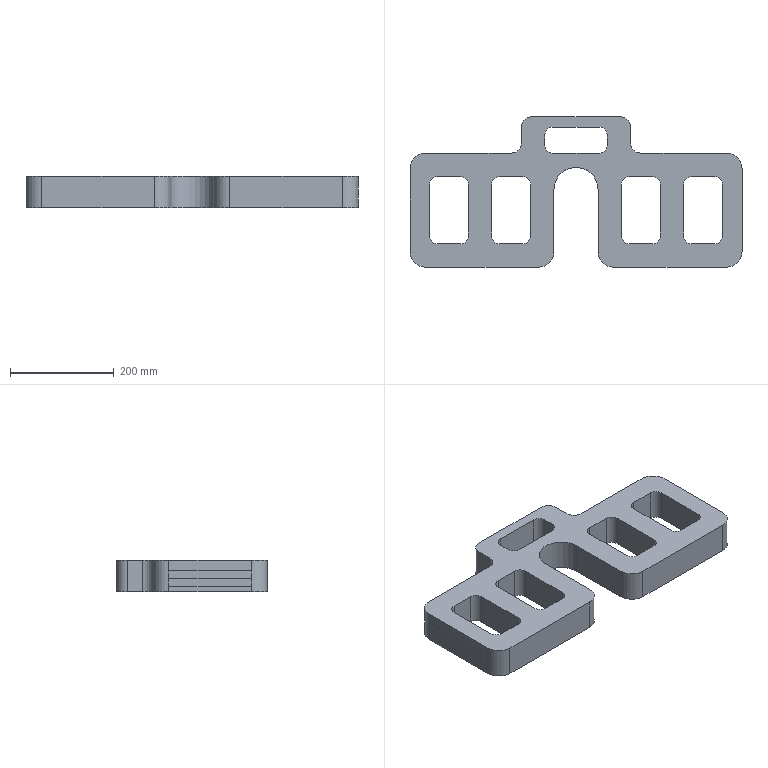Part | SolidWorks | features Fillet 2, Extrusion 1, ICE 1, MirrorPattern 1, PLine 1 | 1 solid | 70 faces | box 640 x 290 x 60 mm | volume 5683176 mm3 | plane 39 | cylinder 31 | commonest cylinder face diameters 30 x20 60 x6 40 x4 85 x1